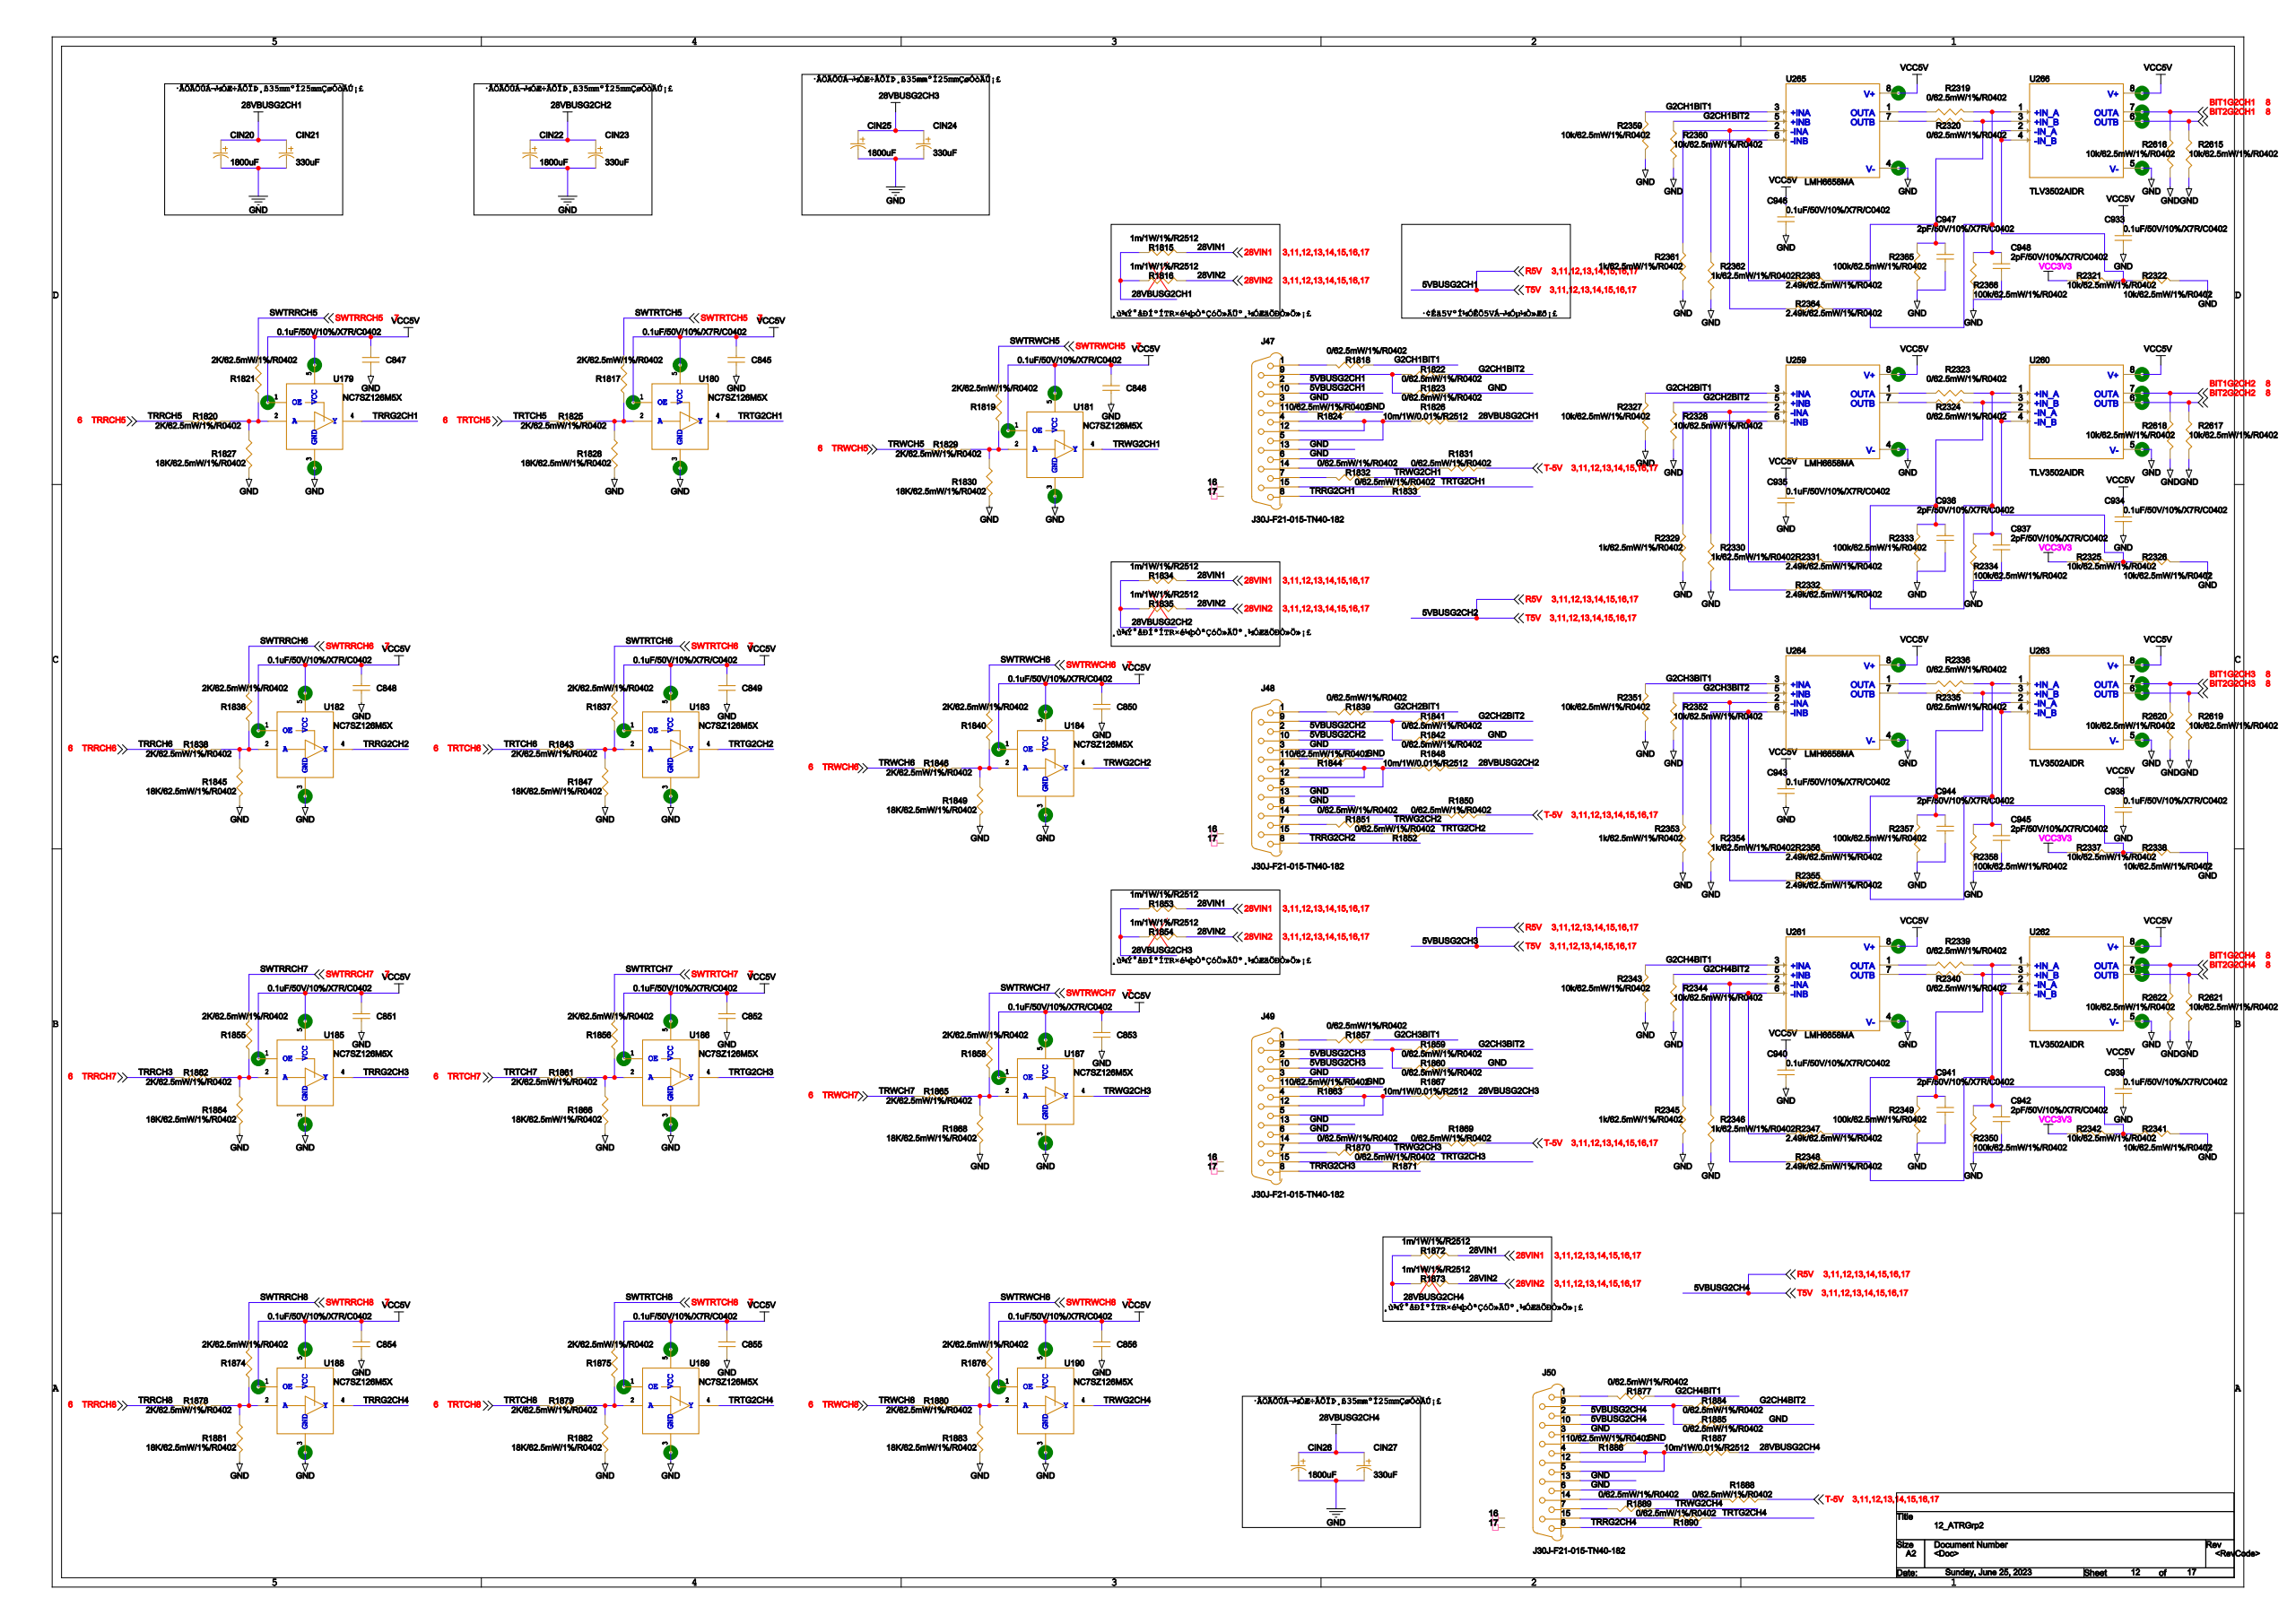Circuit board | Cadence Allegro | 1997 parts | 1536 nets | one sheet of the schematic
Parts on this sheet (reference | value | footprint):
C845 | 0.1uF/50V/10%/X7R/C0402 | 0402
C846 | 0.1uF/50V/10%/X7R/C0402 | 0402
C847 | 0.1uF/50V/10%/X7R/C0402 | 0402
C848 | 0.1uF/50V/10%/X7R/C0402 | 0402
C849 | 0.1uF/50V/10%/X7R/C0402 | 0402
C850 | 0.1uF/50V/10%/X7R/C0402 | 0402
C851 | 0.1uF/50V/10%/X7R/C0402 | 0402
C852 | 0.1uF/50V/10%/X7R/C0402 | 0402
C853 | 0.1uF/50V/10%/X7R/C0402 | 0402
C854 | 0.1uF/50V/10%/X7R/C0402 | 0402
C855 | 0.1uF/50V/10%/X7R/C0402 | 0402
C856 | 0.1uF/50V/10%/X7R/C0402 | 0402
C933 | 0.1uF/50V/10%/X7R/C0402 | 0402
C934 | 0.1uF/50V/10%/X7R/C0402 | 0402
C936 | 2pF/50V/10%/X7R/C0402 | 0402
C937 | 2pF/50V/10%/X7R/C0402 | 0402
C938 | 0.1uF/50V/10%/X7R/C0402 | 0402
C939 | 0.1uF/50V/10%/X7R/C0402 | 0402
C941 | 2pF/50V/10%/X7R/C0402 | 0402
C942 | 2pF/50V/10%/X7R/C0402 | 0402
C944 | 2pF/50V/10%/X7R/C0402 | 0402
C945 | 2pF/50V/10%/X7R/C0402 | 0402
C947 | 2pF/50V/10%/X7R/C0402 | 0402
C948 | 2pF/50V/10%/X7R/C0402 | 0402
CIN20 | ECF1HM182M27OTPO | AP-SMD_BD18-L27-W6_6-LS7_21
CIN21 | ECF1JM331G20OTPO | AP-SMD_BD10-L20-W6_6-LS7_21
CIN22 | ECF1HM182M27OTPO | AP-SMD_BD18-L27-W6_6-LS7_21
CIN23 | ECF1JM331G20OTPO | AP-SMD_BD10-L20-W6_6-LS7_21
CIN24 | ECF1JM331G20OTPO | AP-SMD_BD10-L20-W6_6-LS7_21
CIN25 | ECF1HM182M27OTPO | AP-SMD_BD18-L27-W6_6-LS7_21
CIN26 | ECF1HM182M27OTPO | AP-SMD_BD18-L27-W6_6-LS7_21
CIN27 | ECF1JM331G20OTPO | AP-SMD_BD10-L20-W6_6-LS7_21
J47 | J30J-F21-015-TN40-182 | J30J-F21-015-TN40-182
J48 | J30J-F21-015-TN40-182 | J30J-F21-015-TN40-182
J49 | J30J-F21-015-TN40-182 | J30J-F21-015-TN40-182
J50 | J30J-F21-015-TN40-182 | J30J-F21-015-TN40-182
R1815 | 1m/1W/1%/R2512 | 2512
R1816 | 1m/1W/1%/R2512 | 2512
R1817 | 2K/62.5mW/1%/R0402 | 0402
R1818 | 0/62.5mW/1%/R0402 | 0402
R1819 | 2K/62.5mW/1%/R0402 | 0402
R1820 | 2K/62.5mW/1%/R0402 | 0402
R1821 | 2K/62.5mW/1%/R0402 | 0402
R1822 | 0/62.5mW/1%/R0402 | 0402
R1823 | 0/62.5mW/1%/R0402 | 0402
R1824 | 0/62.5mW/1%/R0402 | 0402
R1825 | 2K/62.5mW/1%/R0402 | 0402
R1826 | 10m/1W/0.01%/R2512 | 2512
R1827 | 18K/62.5mW/1%/R0402 | 0402
R1828 | 18K/62.5mW/1%/R0402 | 0402
R1829 | 2K/62.5mW/1%/R0402 | 0402
R1830 | 18K/62.5mW/1%/R0402 | 0402
R1831 | 0/62.5mW/1%/R0402 | 0402
R1832 | 0/62.5mW/1%/R0402 | 0402
R1833 | 0/62.5mW/1%/R0402 | 0402
R1834 | 1m/1W/1%/R2512 | 2512
R1835 | 1m/1W/1%/R2512 | 2512
R1836 | 2K/62.5mW/1%/R0402 | 0402
R1837 | 2K/62.5mW/1%/R0402 | 0402
R1838 | 2K/62.5mW/1%/R0402 | 0402
R1839 | 0/62.5mW/1%/R0402 | 0402
R1840 | 2K/62.5mW/1%/R0402 | 0402
R1841 | 0/62.5mW/1%/R0402 | 0402
R1842 | 0/62.5mW/1%/R0402 | 0402
R1843 | 2K/62.5mW/1%/R0402 | 0402
R1844 | 0/62.5mW/1%/R0402 | 0402
R1845 | 18K/62.5mW/1%/R0402 | 0402
R1846 | 2K/62.5mW/1%/R0402 | 0402
R1847 | 18K/62.5mW/1%/R0402 | 0402
R1848 | 10m/1W/0.01%/R2512 | 2512
R1849 | 18K/62.5mW/1%/R0402 | 0402
R1850 | 0/62.5mW/1%/R0402 | 0402
R1851 | 0/62.5mW/1%/R0402 | 0402
R1852 | 0/62.5mW/1%/R0402 | 0402
R1853 | 1m/1W/1%/R2512 | 2512
R1854 | 1m/1W/1%/R2512 | 2512
R1855 | 2K/62.5mW/1%/R0402 | 0402
R1856 | 2K/62.5mW/1%/R0402 | 0402
R1857 | 0/62.5mW/1%/R0402 | 0402
R1858 | 2K/62.5mW/1%/R0402 | 0402
R1859 | 0/62.5mW/1%/R0402 | 0402
R1860 | 0/62.5mW/1%/R0402 | 0402
R1861 | 2K/62.5mW/1%/R0402 | 0402
R1862 | 2K/62.5mW/1%/R0402 | 0402
R1863 | 0/62.5mW/1%/R0402 | 0402
R1864 | 18K/62.5mW/1%/R0402 | 0402
R1865 | 2K/62.5mW/1%/R0402 | 0402
R1866 | 18K/62.5mW/1%/R0402 | 0402
R1867 | 10m/1W/0.01%/R2512 | 2512
R1868 | 18K/62.5mW/1%/R0402 | 0402
R1869 | 0/62.5mW/1%/R0402 | 0402
R1870 | 0/62.5mW/1%/R0402 | 0402
R1871 | 0/62.5mW/1%/R0402 | 0402
R1872 | 1m/1W/1%/R2512 | 2512
R1873 | 1m/1W/1%/R2512 | 2512
R1874 | 2K/62.5mW/1%/R0402 | 0402
R1875 | 2K/62.5mW/1%/R0402 | 0402
R1876 | 2K/62.5mW/1%/R0402 | 0402
R1877 | 0/62.5mW/1%/R0402 | 0402
R1878 | 2K/62.5mW/1%/R0402 | 0402
R1879 | 2K/62.5mW/1%/R0402 | 0402
R1880 | 2K/62.5mW/1%/R0402 | 0402
R1881 | 18K/62.5mW/1%/R0402 | 0402
R1882 | 18K/62.5mW/1%/R0402 | 0402
R1883 | 18K/62.5mW/1%/R0402 | 0402
R1884 | 0/62.5mW/1%/R0402 | 0402
R1885 | 0/62.5mW/1%/R0402 | 0402
R1886 | 0/62.5mW/1%/R0402 | 0402
R1887 | 10m/1W/0.01%/R2512 | 2512
R1888 | 0/62.5mW/1%/R0402 | 0402
R1889 | 0/62.5mW/1%/R0402 | 0402
R1890 | 0/62.5mW/1%/R0402 | 0402
R2319 | 0/62.5mW/1%/R0402 | 0402
R2320 | 0/62.5mW/1%/R0402 | 0402
R2321 | 10k/62.5mW/1%/R0402 | 0402
R2322 | 10k/62.5mW/1%/R0402 | 0402
R2323 | 0/62.5mW/1%/R0402 | 0402
R2324 | 0/62.5mW/1%/R0402 | 0402
R2325 | 10k/62.5mW/1%/R0402 | 0402
R2326 | 10k/62.5mW/1%/R0402 | 0402
R2327 | 10k/62.5mW/1%/R0402 | 0402
R2328 | 10k/62.5mW/1%/R0402 | 0402
R2329 | 1K/62.5mW/1%/R0402 | 0402
R2330 | 1K/62.5mW/1%/R0402 | 0402
R2332 | 2.49k/62.5mW/1%/R0402 | 0402
R2333 | 100k/62.5mW/1%/R0402 | 0402
R2334 | 100k/62.5mW/1%/R0402 | 0402
R2335 | 0/62.5mW/1%/R0402 | 0402
R2336 | 0/62.5mW/1%/R0402 | 0402
R2337 | 10k/62.5mW/1%/R0402 | 0402
R2338 | 10k/62.5mW/1%/R0402 | 0402
R2339 | 0/62.5mW/1%/R0402 | 0402
R2340 | 0/62.5mW/1%/R0402 | 0402
R2341 | 10k/62.5mW/1%/R0402 | 0402
R2342 | 10k/62.5mW/1%/R0402 | 0402
R2343 | 10k/62.5mW/1%/R0402 | 0402
R2344 | 10k/62.5mW/1%/R0402 | 0402
R2345 | 1K/62.5mW/1%/R0402 | 0402
R2346 | 1K/62.5mW/1%/R0402 | 0402
R2348 | 2.49k/62.5mW/1%/R0402 | 0402
R2349 | 100k/62.5mW/1%/R0402 | 0402
R2350 | 100k/62.5mW/1%/R0402 | 0402
R2351 | 10k/62.5mW/1%/R0402 | 0402
R2352 | 10k/62.5mW/1%/R0402 | 0402
R2353 | 1K/62.5mW/1%/R0402 | 0402
R2354 | 1K/62.5mW/1%/R0402 | 0402
R2355 | 2.49k/62.5mW/1%/R0402 | 0402
R2356 | 2.49k/62.5mW/1%/R0402 | 0402
R2357 | 100k/62.5mW/1%/R0402 | 0402
R2358 | 100k/62.5mW/1%/R0402 | 0402
R2359 | 10k/62.5mW/1%/R0402 | 0402
R2360 | 10k/62.5mW/1%/R0402 | 0402
R2361 | 1K/62.5mW/1%/R0402 | 0402
R2362 | 1K/62.5mW/1%/R0402 | 0402
R2364 | 2.49k/62.5mW/1%/R0402 | 0402
R2365 | 100k/62.5mW/1%/R0402 | 0402
R2366 | 100k/62.5mW/1%/R0402 | 0402
R2615 | 10k/62.5mW/1%/R0402 | 0402
R2616 | 10k/62.5mW/1%/R0402 | 0402
R2617 | 10k/62.5mW/1%/R0402 | 0402
R2618 | 10k/62.5mW/1%/R0402 | 0402
R2619 | 10k/62.5mW/1%/R0402 | 0402
R2620 | 10k/62.5mW/1%/R0402 | 0402
R2621 | 10k/62.5mW/1%/R0402 | 0402
R2622 | 10k/62.5mW/1%/R0402 | 0402
U179 | NC7SZ126M5X | SOT-23-5
U180 | NC7SZ126M5X | SOT-23-5
U181 | NC7SZ126M5X | SOT-23-5
U182 | NC7SZ126M5X | SOT-23-5
U183 | NC7SZ126M5X | SOT-23-5
U184 | NC7SZ126M5X | SOT-23-5
U185 | NC7SZ126M5X | SOT-23-5
U186 | NC7SZ126M5X | SOT-23-5
U187 | NC7SZ126M5X | SOT-23-5
U188 | NC7SZ126M5X | SOT-23-5
U189 | NC7SZ126M5X | SOT-23-5
U190 | NC7SZ126M5X | SOT-23-5
U259 | LMH6658MA | SOIC127P599X175-8N
U261 | LMH6658MA | SOIC127P599X175-8N
U263 | TLV3502AIDR | SOIC127P599X175-8N
U265 | LMH6658MA | SOIC127P599X175-8N
Nets of these parts (net: part-pin ...):
3.3V: R2321-1 R2325-1 R2337-1 R2342-1
AGND: C845-2 C846-2 C847-2 C848-2 C849-2 C850-2 C851-2 C852-2 C853-2 C854-2 C855-2 C856-2 C933-2 C934-2 C936-2 C937-2 C938-2 C939-2 C941-2 C942-2 C944-2 C945-2 C947-2 C948-2 CIN20-2 CIN21-2 CIN22-2 CIN23-2 CIN24-2 CIN25-2 CIN26-2 CIN27-2 J47-3 J47-6 J47-13 J48-3 J48-6 J48-13 J49-3 J49-6 J49-13 J50-3 J50-6 J50-13 R1823-1 R1824-1 R1827-1 R1828-1 R1830-1 R1842-1 R1844-1 R1845-1 R1847-1 R1849-1 R1860-1 R1863-1 R1864-1 R1866-1 R1868-1 R1881-1 R1882-1 R1883-1 R1885-1 R1886-1 R2322-2 R2326-2 R2327-2 R2328-2 R2329-2 R2330-2 R2333-2 R2334-2 R2338-2 R2341-2 R2343-2 R2344-2 R2345-2 R2346-2 R2349-2 R2350-2 R2351-2 R2352-2 R2353-2 R2354-2 R2357-2 R2358-2 R2359-2 R2360-2 R2361-2 R2362-2 R2365-2 R2366-2 R2615-2 R2616-2 R2617-2 R2618-2 R2619-2 R2620-2 R2621-2 R2622-2 U179-3 U180-3 U181-3 U182-3 U183-3 U184-3 U185-3 U186-3 U187-3 U188-3 U189-3 U190-3 U259-4 U261-4 U263-5 U265-4
VCC5V: C845-1 C846-1 C847-1 C848-1 C849-1 C850-1 C851-1 C852-1 C853-1 C854-1 C855-1 C856-1 C933-1 C934-1 C938-1 C939-1 U179-1 U179-5 U180-1 U180-5 U181-1 U181-5 U182-1 U182-5 U183-1 U183-5 U184-1 U184-5 U185-1 U185-5 U186-1 U186-5 U187-1 U187-5 U188-1 U188-5 U189-1 U189-5 U190-1 U190-5 U259-8 U261-8 U263-8 U265-8
N24395982: R2330-1 U259-6
N24395992: C936-1 R2324-2 R2333-1
N24395970: R2329-1 R2332-1 U259-2
N24395990: C937-1 R2323-2 R2332-2 R2334-1
N24396536: R2346-1 U261-6
N24396546: C941-1 R2340-2 R2349-1
N24396524: R2345-1 R2348-1 U261-2
N24396544: C942-1 R2339-2 R2348-2 R2350-1
N24396348: R2353-1 R2355-1
N24396364: C945-1 R2336-2 R2355-2 R2358-1 U263-1
N24396352: R2354-1 R2356-1
N24396366: C944-1 R2335-2 R2356-2 R2357-1 U263-3
N24395802: R2362-1 U265-6
N24395812: C947-1 R2320-2 R2365-1
N24395798: R2361-1 R2364-1 U265-2
N24395810: C948-1 R2319-2 R2364-2 R2366-1
G2CH2BIT1: R1839-1 R2327-1 U259-3
G2CH2BIT2: R1841-1 R2328-1 U259-5
N24395986: R2323-1 U259-1
N24395988: R2324-1 U259-7
G2CH4BIT1: R1877-1 R2343-1 U261-3
G2CH4BIT2: R1884-1 R2344-1 U261-5
N24396540: R2339-1 U261-1
N24396542: R2340-1 U261-7
G2CH3BIT1: R1857-1 R2351-1
G2CH3BIT2: R1859-1 R2352-1
N24396360: R2336-1
N24396362: R2335-1
G2CH1BIT1: R1818-1 R2359-1 U265-3
G2CH1BIT2: R1822-1 R2360-1 U265-5
N24395806: R2319-1 U265-1
N24395808: R2320-1 U265-7
N24396044: R2325-2 R2326-1
BIT1G2CH2: R2618-1
BIT2G2CH2: R2617-1
N24396598: R2341-1 R2342-2
BIT1G2CH4: R2622-1
BIT2G2CH4: R2621-1
N24396418: R2337-2 R2338-1 U263-2 U263-4
BIT1G2CH3: R2620-1 U263-7
BIT2G2CH3: R2619-1 U263-6
N24395864: R2321-2 R2322-1
BIT1G2CH1: R2616-1
BIT2G2CH1: R2615-1
R5V: J47-2 J47-10 J48-2 J48-10 J49-2 J49-10 J50-2 J50-10
N23722815: J47-1 R1818-2
N23722828: J47-11 R1824-2
N23722830: J47-4 J47-5 J47-12 R1826-1
N23722842: J47-14 R1831-2
N23722846: J47-15 R1833-2
N23722844: J47-7 R1832-2
TRRG2CH1: J47-8 U179-4
N23722817: J47-9 R1822-2 R1823-2
N23723374: J48-1 R1839-2
N23723387: J48-11 R1844-2
N23723389: J48-4 J48-5 J48-12 R1848-1
N23723401: J48-14 R1850-2
N23723405: J48-15 R1852-2
N23723403: J48-7 R1851-2
TRRG2CH2: J48-8 U182-4
N23723376: J48-9 R1841-2 R1842-2
N23724001: J49-1 R1857-2
N23724014: J49-11 R1863-2
N23724016: J49-4 J49-5 J49-12 R1867-1
N23724028: J49-14 R1869-2
N23724032: J49-15 R1871-2
N23724030: J49-7 R1870-2
TRRG2CH3: J49-8 U185-4
N23724003: J49-9 R1859-2 R1860-2
N23724633: J50-1 R1877-2
N23724646: J50-11 R1886-2
N23724648: J50-4 J50-5 J50-12 R1887-1
N23724660: J50-14 R1888-2
N23724664: J50-15 R1890-2
N23724662: J50-7 R1889-2
TRRG2CH4: J50-8 U188-4
N23724635: J50-9 R1884-2 R1885-2
28VIN1: R1815-2 R1834-2 R1853-2 R1872-2
T-5V: R1831-1 R1850-1 R1869-1 R1888-1
28VIN2: R1816-2 R1835-2 R1854-2 R1873-2
28VBUSG2CH1: CIN20-1 CIN21-1 R1815-1 R1816-1 R1826-2
28VBUSG2CH2: CIN22-1 CIN23-1 R1834-1 R1835-1 R1848-2
28VBUSG2CH3: CIN24-1 CIN25-1 R1853-1 R1854-1 R1867-2
28VBUSG2CH4: CIN26-1 CIN27-1 R1872-1 R1873-1 R1887-2
SWTRTCH5: R1817-1
N24002951: R1817-2 R1825-2 R1828-2 U180-2
SWTRWCH5: R1819-1
N24003439: R1819-2 R1829-2 R1830-2 U181-2
TRRCH5: R1820-1
N24003931: R1820-2 R1821-2 R1827-2 U179-2
SWTRRCH5: R1821-1
TRTCH5: R1825-1
TRWCH5: R1829-1
SWTRRCH6: R1836-1
N24004049: R1836-2 R1838-2 R1845-2 U182-2
SWTRTCH6: R1837-1
N24003069: R1837-2 R1843-2 R1847-2 U183-2
TRRCH6: R1838-1
SWTRWCH6: R1840-1
N24003561: R1840-2 R1846-2 R1849-2 U184-2
TRTCH6: R1843-1
TRWCH6: R1846-1
SWTRRCH7: R1855-1
N24004175: R1855-2 R1862-2 R1864-2 U185-2
SWTRTCH7: R1856-1
N24003195: R1856-2 R1861-2 R1866-2 U186-2
SWTRWCH7: R1858-1
N24003683: R1858-2 R1865-2 R1868-2 U187-2
TRTCH7: R1861-1
TRRCH7: R1862-1
TRWCH7: R1865-1
SWTRRCH8: R1874-1
N24004293: R1874-2 R1878-2 R1881-2 U188-2
SWTRTCH8: R1875-1
N24003317: R1875-2 R1879-2 R1882-2 U189-2
SWTRWCH8: R1876-1
N24003805: R1876-2 R1880-2 R1883-2 U190-2
TRRCH8: R1878-1
TRTCH8: R1879-1
TRWCH8: R1880-1
TRTG2CH1: R1833-1 U180-4
TRWG2CH1: R1832-1 U181-4
TRTG2CH2: R1852-1 U183-4
TRWG2CH2: R1851-1 U184-4
TRTG2CH3: R1871-1 U186-4
TRWG2CH3: R1870-1 U187-4
TRTG2CH4: R1890-1 U189-4
TRWG2CH4: R1889-1 U190-4